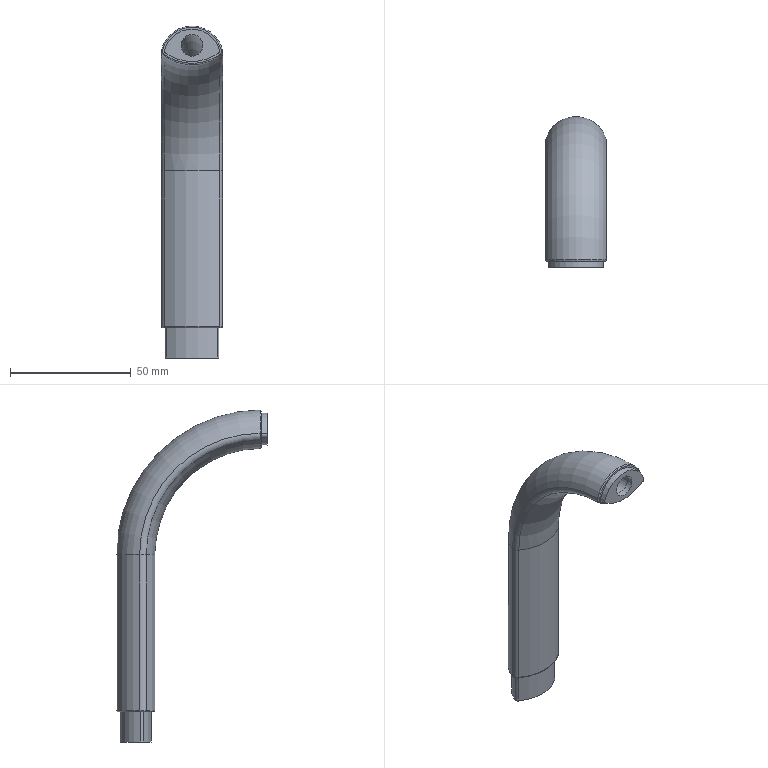Part | NX | features DATUM_CSYS 5, SKETCH 4, BLEND 2, EXTRUDE 2, SCALE 1, SWP104 1 | 1 solid | 31 faces | box 25.275 x 62.5 x 137.498 mm | volume 37253 mm3 | cylinder 14 | torus 9 | plane 4 | spline 4 | commonest cylinder face diameters 2 x2 2.5 x2 5 x2 9 x2 23 x1 23.5 x1
STEP:
#1=CARTESIAN_POINT('',(-12.068,0.2563,0.));
#2=VERTEX_POINT('',#1);
#3=CARTESIAN_POINT('',(12.068,0.2563,0.));
#4=VERTEX_POINT('',#3);
#5=CARTESIAN_POINT('',(0.,-3.,0.));
#6=DIRECTION('',(0.,0.,1.));
#7=DIRECTION('',(1.,0.,0.));
#8=AXIS2_PLACEMENT_3D('',#5,#6,#7);
#9=CIRCLE('',#8,12.5);
#10=EDGE_CURVE('',#2,#4,#9,.F.);
#11=ORIENTED_EDGE('',*,*,#10,.T.);
#12=CARTESIAN_POINT('',(11.296,-1.895,0.));
#13=VERTEX_POINT('',#12);
#14=CARTESIAN_POINT('',(10.137,-0.2647,0.));
#15=DIRECTION('',(0.,0.,1.));
#16=DIRECTION('',(1.,0.,0.));
#17=AXIS2_PLACEMENT_3D('',#14,#15,#16);
#18=CIRCLE('',#17,2.);
#19=EDGE_CURVE('',#4,#13,#18,.F.);
#20=ORIENTED_EDGE('',*,*,#19,.T.);
#21=CARTESIAN_POINT('',(-11.296,-1.895,0.));
#22=VERTEX_POINT('',#21);
#23=CARTESIAN_POINT('',(0.,14.,0.));
#24=DIRECTION('',(0.,0.,1.));
#25=DIRECTION('',(1.,0.,0.));
#26=AXIS2_PLACEMENT_3D('',#23,#24,#25);
#27=CIRCLE('',#26,19.5);
#28=EDGE_CURVE('',#13,#22,#27,.F.);
#29=ORIENTED_EDGE('',*,*,#28,.T.);
#30=CARTESIAN_POINT('',(-10.137,-0.2647,0.));
#31=DIRECTION('',(0.,0.,1.));
#32=DIRECTION('',(1.,0.,0.));
#33=AXIS2_PLACEMENT_3D('',#30,#31,#32);
#34=CIRCLE('',#33,2.);
#35=EDGE_CURVE('',#22,#2,#34,.F.);
#36=ORIENTED_EDGE('',*,*,#35,.T.);
#37=EDGE_LOOP('',(#11,#20,#29,#36));
#38=FACE_BOUND('',#37,.T.);
#39=CARTESIAN_POINT('',(-10.717,-1.08,0.));
#40=VERTEX_POINT('',#39);
#41=CARTESIAN_POINT('',(-11.103,-0.004202,0.));
#42=VERTEX_POINT('',#41);
#43=CARTESIAN_POINT('',(-10.137,-0.2647,0.));
#44=DIRECTION('',(0.,0.,-1.));
#45=DIRECTION('',(1.,0.,0.));
#46=AXIS2_PLACEMENT_3D('',#43,#44,#45);
#47=CIRCLE('',#46,1.);
#48=EDGE_CURVE('',#40,#42,#47,.T.);
#49=ORIENTED_EDGE('',*,*,#48,.F.);
#50=CARTESIAN_POINT('',(10.717,-1.08,0.));
#51=VERTEX_POINT('',#50);
#52=CARTESIAN_POINT('',(0.,14.,0.));
#53=DIRECTION('',(0.,0.,-1.));
#54=DIRECTION('',(1.,0.,0.));
#55=AXIS2_PLACEMENT_3D('',#52,#53,#54);
#56=CIRCLE('',#55,18.5);
#57=EDGE_CURVE('',#51,#40,#56,.T.);
#58=ORIENTED_EDGE('',*,*,#57,.F.);
#59=CARTESIAN_POINT('',(11.103,-0.004202,0.));
#60=VERTEX_POINT('',#59);
#61=CARTESIAN_POINT('',(10.137,-0.2647,0.));
#62=DIRECTION('',(0.,0.,-1.));
#63=DIRECTION('',(1.,0.,0.));
#64=AXIS2_PLACEMENT_3D('',#61,#62,#63);
#65=CIRCLE('',#64,1.);
#66=EDGE_CURVE('',#60,#51,#65,.T.);
#67=ORIENTED_EDGE('',*,*,#66,.F.);
#68=CARTESIAN_POINT('',(0.,-3.,0.));
#69=DIRECTION('',(0.,0.,-1.));
#70=DIRECTION('',(1.,0.,0.));
#71=AXIS2_PLACEMENT_3D('',#68,#69,#70);
#72=CIRCLE('',#71,11.5);
#73=EDGE_CURVE('',#42,#60,#72,.T.);
#74=ORIENTED_EDGE('',*,*,#73,.F.);
#75=EDGE_LOOP('',(#49,#58,#67,#74));
#76=FACE_BOUND('',#75,.T.);
#77=CARTESIAN_POINT('',(5.069,-1.632,0.));
#78=DIRECTION('',(0.,0.,1.));
#79=DIRECTION('',(1.,0.,0.));
#80=AXIS2_PLACEMENT_3D('',#77,#78,#79);
#81=PLANE('',#80);
#82=ADVANCED_FACE('',(#38,#76),#81,.F.);
#83=CARTESIAN_POINT('',(-12.551,0.3866,65.));
#84=VERTEX_POINT('',#83);
#85=CARTESIAN_POINT('',(-12.551,-49.499,115.384));
#86=VERTEX_POINT('',#85);
#87=CARTESIAN_POINT('',(-12.551,-50.,65.));
#88=DIRECTION('',(1.,0.,0.));
#89=DIRECTION('',(0.,0.,-1.));
#90=AXIS2_PLACEMENT_3D('',#87,#88,#89);
#91=CIRCLE('',#90,50.387);
#92=EDGE_CURVE('',#84,#86,#91,.T.);
#93=ORIENTED_EDGE('',*,*,#92,.T.);
#94=CARTESIAN_POINT('',(12.551,-49.499,115.384));
#95=VERTEX_POINT('',#94);
#96=CARTESIAN_POINT('',(-12.551,-49.499,115.384));
#97=CARTESIAN_POINT('',(-11.807,-49.498,118.142));
#98=CARTESIAN_POINT('',(-8.48,-49.496,123.077));
#99=CARTESIAN_POINT('',(-0.002474,-49.496,125.957));
#100=CARTESIAN_POINT('',(8.472,-49.496,123.084));
#101=CARTESIAN_POINT('',(11.807,-49.498,118.142));
#102=CARTESIAN_POINT('',(12.551,-49.499,115.384));
#103=B_SPLINE_CURVE_WITH_KNOTS('',3,(#96,#97,#98,#99,#100,#101,#102),.UNSPECIFIED.,.F.,.F.,(4,1,1,1,4),(0.,0.0085,0.017,0.0255,0.034),.UNSPECIFIED.);
#104=EDGE_CURVE('',#86,#95,#103,.T.);
#105=ORIENTED_EDGE('',*,*,#104,.T.);
#106=CARTESIAN_POINT('',(12.551,0.3866,65.));
#107=VERTEX_POINT('',#106);
#108=CARTESIAN_POINT('',(12.551,-50.,65.));
#109=DIRECTION('',(1.,0.,0.));
#110=DIRECTION('',(0.,0.,-1.));
#111=AXIS2_PLACEMENT_3D('',#108,#109,#110);
#112=CIRCLE('',#111,50.387);
#113=EDGE_CURVE('',#107,#95,#112,.T.);
#114=ORIENTED_EDGE('',*,*,#113,.F.);
#115=CARTESIAN_POINT('',(0.,-3.,65.));
#116=DIRECTION('',(0.,0.,1.));
#117=DIRECTION('',(1.,0.,0.));
#118=AXIS2_PLACEMENT_3D('',#115,#116,#117);
#119=CIRCLE('',#118,13.);
#120=EDGE_CURVE('',#107,#84,#119,.T.);
#121=ORIENTED_EDGE('',*,*,#120,.T.);
#122=EDGE_LOOP('',(#93,#105,#114,#121));
#123=FACE_BOUND('',#122,.T.);
#124=CARTESIAN_POINT('',(0.,-50.,65.));
#125=DIRECTION('',(1.,0.,0.));
#126=DIRECTION('',(0.,0.,-1.));
#127=AXIS2_PLACEMENT_3D('',#124,#125,#126);
#128=TOROIDAL_SURFACE('',#127,47.,13.);
#129=ADVANCED_FACE('',(#123),#128,.T.);
#130=CARTESIAN_POINT('',(-11.586,-2.303,65.));
#131=VERTEX_POINT('',#130);
#132=CARTESIAN_POINT('',(-11.586,-49.504,112.695));
#133=VERTEX_POINT('',#132);
#134=CARTESIAN_POINT('',(-11.586,-50.,65.));
#135=DIRECTION('',(1.,0.,0.));
#136=DIRECTION('',(0.,0.,-1.));
#137=AXIS2_PLACEMENT_3D('',#134,#135,#136);
#138=CIRCLE('',#137,47.697);
#139=EDGE_CURVE('',#131,#133,#138,.T.);
#140=ORIENTED_EDGE('',*,*,#139,.T.);
#141=CARTESIAN_POINT('',(-11.586,-49.504,112.695));
#142=CARTESIAN_POINT('',(-12.419,-49.503,113.287));
#143=CARTESIAN_POINT('',(-12.817,-49.501,114.397));
#144=CARTESIAN_POINT('',(-12.551,-49.499,115.384));
#145=B_SPLINE_CURVE_WITH_KNOTS('',3,(#141,#142,#143,#144),.UNSPECIFIED.,.F.,.F.,(4,4),(0.,0.003051),.UNSPECIFIED.);
#146=EDGE_CURVE('',#133,#86,#145,.T.);
#147=ORIENTED_EDGE('',*,*,#146,.T.);
#148=ORIENTED_EDGE('',*,*,#92,.F.);
#149=CARTESIAN_POINT('',(-10.137,-0.2647,65.));
#150=DIRECTION('',(0.,0.,1.));
#151=DIRECTION('',(1.,0.,0.));
#152=AXIS2_PLACEMENT_3D('',#149,#150,#151);
#153=CIRCLE('',#152,2.5);
#154=EDGE_CURVE('',#84,#131,#153,.T.);
#155=ORIENTED_EDGE('',*,*,#154,.T.);
#156=EDGE_LOOP('',(#140,#147,#148,#155));
#157=FACE_BOUND('',#156,.T.);
#158=CARTESIAN_POINT('',(-10.137,-50.,65.));
#159=DIRECTION('',(1.,0.,0.));
#160=DIRECTION('',(0.,0.,-1.));
#161=AXIS2_PLACEMENT_3D('',#158,#159,#160);
#162=TOROIDAL_SURFACE('',#161,49.735,2.5);
#163=ADVANCED_FACE('',(#157),#162,.T.);
#164=CARTESIAN_POINT('',(11.586,-2.303,65.));
#165=VERTEX_POINT('',#164);
#166=CARTESIAN_POINT('',(11.586,-49.504,112.695));
#167=VERTEX_POINT('',#166);
#168=CARTESIAN_POINT('',(11.586,-50.,65.));
#169=DIRECTION('',(1.,0.,0.));
#170=DIRECTION('',(0.,0.,-1.));
#171=AXIS2_PLACEMENT_3D('',#168,#169,#170);
#172=CIRCLE('',#171,47.697);
#173=EDGE_CURVE('',#165,#167,#172,.T.);
#174=ORIENTED_EDGE('',*,*,#173,.T.);
#175=CARTESIAN_POINT('',(11.586,-49.504,112.695));
#176=CARTESIAN_POINT('',(8.204,-49.505,110.291));
#177=CARTESIAN_POINT('',(-0.002573,-49.506,107.703));
#178=CARTESIAN_POINT('',(-8.204,-49.505,110.291));
#179=CARTESIAN_POINT('',(-11.586,-49.504,112.695));
#180=B_SPLINE_CURVE_WITH_KNOTS('',3,(#175,#176,#177,#178,#179),.UNSPECIFIED.,.F.,.F.,(4,1,4),(0.,0.01237,0.02474),.UNSPECIFIED.);
#181=EDGE_CURVE('',#167,#133,#180,.T.);
#182=ORIENTED_EDGE('',*,*,#181,.T.);
#183=ORIENTED_EDGE('',*,*,#139,.F.);
#184=CARTESIAN_POINT('',(0.,14.,65.));
#185=DIRECTION('',(0.,0.,1.));
#186=DIRECTION('',(1.,0.,0.));
#187=AXIS2_PLACEMENT_3D('',#184,#185,#186);
#188=CIRCLE('',#187,20.);
#189=EDGE_CURVE('',#131,#165,#188,.T.);
#190=ORIENTED_EDGE('',*,*,#189,.T.);
#191=EDGE_LOOP('',(#174,#182,#183,#190));
#192=FACE_BOUND('',#191,.T.);
#193=CARTESIAN_POINT('',(0.,-50.,65.));
#194=DIRECTION('',(1.,0.,0.));
#195=DIRECTION('',(0.,0.,-1.));
#196=AXIS2_PLACEMENT_3D('',#193,#194,#195);
#197=TOROIDAL_SURFACE('',#196,64.,20.);
#198=ADVANCED_FACE('',(#192),#197,.T.);
#199=ORIENTED_EDGE('',*,*,#113,.T.);
#200=CARTESIAN_POINT('',(12.551,-49.499,115.384));
#201=CARTESIAN_POINT('',(12.817,-49.501,114.397));
#202=CARTESIAN_POINT('',(12.419,-49.503,113.287));
#203=CARTESIAN_POINT('',(11.586,-49.504,112.695));
#204=B_SPLINE_CURVE_WITH_KNOTS('',3,(#200,#201,#202,#203),.UNSPECIFIED.,.F.,.F.,(4,4),(0.,0.003051),.UNSPECIFIED.);
#205=EDGE_CURVE('',#95,#167,#204,.T.);
#206=ORIENTED_EDGE('',*,*,#205,.T.);
#207=ORIENTED_EDGE('',*,*,#173,.F.);
#208=CARTESIAN_POINT('',(10.137,-0.2647,65.));
#209=DIRECTION('',(0.,0.,1.));
#210=DIRECTION('',(1.,0.,0.));
#211=AXIS2_PLACEMENT_3D('',#208,#209,#210);
#212=CIRCLE('',#211,2.5);
#213=EDGE_CURVE('',#165,#107,#212,.T.);
#214=ORIENTED_EDGE('',*,*,#213,.T.);
#215=EDGE_LOOP('',(#199,#206,#207,#214));
#216=FACE_BOUND('',#215,.T.);
#217=CARTESIAN_POINT('',(10.137,-50.,65.));
#218=DIRECTION('',(1.,0.,0.));
#219=DIRECTION('',(0.,0.,-1.));
#220=AXIS2_PLACEMENT_3D('',#217,#218,#219);
#221=TOROIDAL_SURFACE('',#220,49.735,2.5);
#222=ADVANCED_FACE('',(#216),#221,.T.);
#223=CARTESIAN_POINT('',(4.5,2.,65.));
#224=VERTEX_POINT('',#223);
#225=CARTESIAN_POINT('',(0.,2.,65.));
#226=DIRECTION('',(0.,0.,1.));
#227=DIRECTION('',(1.,0.,0.));
#228=AXIS2_PLACEMENT_3D('',#225,#226,#227);
#229=CIRCLE('',#228,4.5);
#230=EDGE_CURVE('',#224,#224,#229,.T.);
#231=ORIENTED_EDGE('',*,*,#230,.F.);
#232=EDGE_LOOP('',(#231));
#233=FACE_BOUND('',#232,.T.);
#234=CARTESIAN_POINT('',(4.5,-50.,117.));
#235=VERTEX_POINT('',#234);
#236=CARTESIAN_POINT('',(0.,-50.,117.));
#237=DIRECTION('',(0.,-1.,0.));
#238=DIRECTION('',(1.,0.,0.));
#239=AXIS2_PLACEMENT_3D('',#236,#237,#238);
#240=CIRCLE('',#239,4.5);
#241=EDGE_CURVE('',#235,#235,#240,.T.);
#242=ORIENTED_EDGE('',*,*,#241,.T.);
#243=EDGE_LOOP('',(#242));
#244=FACE_BOUND('',#243,.T.);
#245=CARTESIAN_POINT('',(0.,-50.,65.));
#246=DIRECTION('',(1.,0.,0.));
#247=DIRECTION('',(0.,0.,-1.));
#248=AXIS2_PLACEMENT_3D('',#245,#246,#247);
#249=TOROIDAL_SURFACE('',#248,52.,4.5);
#250=ADVANCED_FACE('',(#233,#244),#249,.F.);
#251=CARTESIAN_POINT('',(11.586,-2.303,0.5));
#252=VERTEX_POINT('',#251);
#253=CARTESIAN_POINT('',(11.586,-2.303,65.));
#254=DIRECTION('',(0.,0.,-1.));
#255=VECTOR('',#254,1000.);
#256=LINE('',#253,#255);
#257=EDGE_CURVE('',#165,#252,#256,.T.);
#258=ORIENTED_EDGE('',*,*,#257,.T.);
#259=CARTESIAN_POINT('',(12.551,0.3866,0.5));
#260=VERTEX_POINT('',#259);
#261=CARTESIAN_POINT('',(10.137,-0.2647,0.5));
#262=DIRECTION('',(0.,0.,1.));
#263=DIRECTION('',(1.,0.,0.));
#264=AXIS2_PLACEMENT_3D('',#261,#262,#263);
#265=CIRCLE('',#264,2.5);
#266=EDGE_CURVE('',#252,#260,#265,.T.);
#267=ORIENTED_EDGE('',*,*,#266,.T.);
#268=CARTESIAN_POINT('',(12.551,0.3866,65.));
#269=DIRECTION('',(0.,0.,-1.));
#270=VECTOR('',#269,1000.);
#271=LINE('',#268,#270);
#272=EDGE_CURVE('',#107,#260,#271,.T.);
#273=ORIENTED_EDGE('',*,*,#272,.F.);
#274=ORIENTED_EDGE('',*,*,#213,.F.);
#275=EDGE_LOOP('',(#258,#267,#273,#274));
#276=FACE_BOUND('',#275,.T.);
#277=CARTESIAN_POINT('',(10.137,-0.2647,65.));
#278=DIRECTION('',(0.,0.,-1.));
#279=DIRECTION('',(-1.,0.,0.));
#280=AXIS2_PLACEMENT_3D('',#277,#278,#279);
#281=CYLINDRICAL_SURFACE('',#280,2.5);
#282=ADVANCED_FACE('',(#276),#281,.T.);
#283=ORIENTED_EDGE('',*,*,#272,.T.);
#284=CARTESIAN_POINT('',(-12.551,0.3866,0.5));
#285=VERTEX_POINT('',#284);
#286=CARTESIAN_POINT('',(0.,-3.,0.5));
#287=DIRECTION('',(0.,0.,1.));
#288=DIRECTION('',(1.,0.,0.));
#289=AXIS2_PLACEMENT_3D('',#286,#287,#288);
#290=CIRCLE('',#289,13.);
#291=EDGE_CURVE('',#260,#285,#290,.T.);
#292=ORIENTED_EDGE('',*,*,#291,.T.);
#293=CARTESIAN_POINT('',(-12.551,0.3866,65.));
#294=DIRECTION('',(0.,0.,-1.));
#295=VECTOR('',#294,1000.);
#296=LINE('',#293,#295);
#297=EDGE_CURVE('',#84,#285,#296,.T.);
#298=ORIENTED_EDGE('',*,*,#297,.F.);
#299=ORIENTED_EDGE('',*,*,#120,.F.);
#300=EDGE_LOOP('',(#283,#292,#298,#299));
#301=FACE_BOUND('',#300,.T.);
#302=CARTESIAN_POINT('',(0.,-3.,65.));
#303=DIRECTION('',(0.,0.,-1.));
#304=DIRECTION('',(-1.,0.,0.));
#305=AXIS2_PLACEMENT_3D('',#302,#303,#304);
#306=CYLINDRICAL_SURFACE('',#305,13.);
#307=ADVANCED_FACE('',(#301),#306,.T.);
#308=ORIENTED_EDGE('',*,*,#297,.T.);
#309=CARTESIAN_POINT('',(-11.586,-2.303,0.5));
#310=VERTEX_POINT('',#309);
#311=CARTESIAN_POINT('',(-10.137,-0.2647,0.5));
#312=DIRECTION('',(0.,0.,1.));
#313=DIRECTION('',(1.,0.,0.));
#314=AXIS2_PLACEMENT_3D('',#311,#312,#313);
#315=CIRCLE('',#314,2.5);
#316=EDGE_CURVE('',#285,#310,#315,.T.);
#317=ORIENTED_EDGE('',*,*,#316,.T.);
#318=CARTESIAN_POINT('',(-11.586,-2.303,65.));
#319=DIRECTION('',(0.,0.,-1.));
#320=VECTOR('',#319,1000.);
#321=LINE('',#318,#320);
#322=EDGE_CURVE('',#131,#310,#321,.T.);
#323=ORIENTED_EDGE('',*,*,#322,.F.);
#324=ORIENTED_EDGE('',*,*,#154,.F.);
#325=EDGE_LOOP('',(#308,#317,#323,#324));
#326=FACE_BOUND('',#325,.T.);
#327=CARTESIAN_POINT('',(-10.137,-0.2647,65.));
#328=DIRECTION('',(0.,0.,-1.));
#329=DIRECTION('',(-1.,0.,0.));
#330=AXIS2_PLACEMENT_3D('',#327,#328,#329);
#331=CYLINDRICAL_SURFACE('',#330,2.5);
#332=ADVANCED_FACE('',(#326),#331,.T.);
#333=ORIENTED_EDGE('',*,*,#230,.T.);
#334=EDGE_LOOP('',(#333));
#335=FACE_BOUND('',#334,.T.);
#336=CARTESIAN_POINT('',(4.5,2.,-12.5));
#337=VERTEX_POINT('',#336);
#338=CARTESIAN_POINT('',(0.,2.,-12.5));
#339=DIRECTION('',(0.,0.,-1.));
#340=DIRECTION('',(1.,0.,0.));
#341=AXIS2_PLACEMENT_3D('',#338,#339,#340);
#342=CIRCLE('',#341,4.5);
#343=EDGE_CURVE('',#337,#337,#342,.T.);
#344=ORIENTED_EDGE('',*,*,#343,.T.);
#345=EDGE_LOOP('',(#344));
#346=FACE_BOUND('',#345,.T.);
#347=CARTESIAN_POINT('',(0.,2.,65.));
#348=DIRECTION('',(0.,0.,-1.));
#349=DIRECTION('',(-1.,0.,0.));
#350=AXIS2_PLACEMENT_3D('',#347,#348,#349);
#351=CYLINDRICAL_SURFACE('',#350,4.5);
#352=ADVANCED_FACE('',(#335,#346),#351,.F.);
#353=ORIENTED_EDGE('',*,*,#322,.T.);
#354=CARTESIAN_POINT('',(0.,14.,0.5));
#355=DIRECTION('',(0.,0.,1.));
#356=DIRECTION('',(1.,0.,0.));
#357=AXIS2_PLACEMENT_3D('',#354,#355,#356);
#358=CIRCLE('',#357,20.);
#359=EDGE_CURVE('',#310,#252,#358,.T.);
#360=ORIENTED_EDGE('',*,*,#359,.T.);
#361=ORIENTED_EDGE('',*,*,#257,.F.);
#362=ORIENTED_EDGE('',*,*,#189,.F.);
#363=EDGE_LOOP('',(#353,#360,#361,#362));
#364=FACE_BOUND('',#363,.T.);
#365=CARTESIAN_POINT('',(0.,14.,65.));
#366=DIRECTION('',(0.,0.,-1.));
#367=DIRECTION('',(-1.,0.,0.));
#368=AXIS2_PLACEMENT_3D('',#365,#366,#367);
#369=CYLINDRICAL_SURFACE('',#368,20.);
#370=ADVANCED_FACE('',(#364),#369,.T.);
#371=CARTESIAN_POINT('',(-11.296,-50.,113.102));
#372=VERTEX_POINT('',#371);
#373=CARTESIAN_POINT('',(11.296,-50.,113.102));
#374=VERTEX_POINT('',#373);
#375=CARTESIAN_POINT('',(-11.296,-50.,113.102));
#376=CARTESIAN_POINT('',(-7.994,-50.,110.756));
#377=CARTESIAN_POINT('',(-0.03503,-50.,108.239));
#378=CARTESIAN_POINT('',(7.994,-50.,110.756));
#379=CARTESIAN_POINT('',(11.296,-50.,113.102));
#380=B_SPLINE_CURVE_WITH_KNOTS('',3,(#375,#376,#377,#378,#379),.UNSPECIFIED.,.F.,.F.,(4,1,4),(0.,0.01198,0.02396),.UNSPECIFIED.);
#381=EDGE_CURVE('',#372,#374,#380,.T.);
#382=ORIENTED_EDGE('',*,*,#381,.T.);
#383=CARTESIAN_POINT('',(12.068,-50.,115.254));
#384=VERTEX_POINT('',#383);
#385=CARTESIAN_POINT('',(11.296,-50.,113.102));
#386=CARTESIAN_POINT('',(11.963,-50.,113.576));
#387=CARTESIAN_POINT('',(12.281,-50.,114.464));
#388=CARTESIAN_POINT('',(12.068,-50.,115.254));
#389=B_SPLINE_CURVE_WITH_KNOTS('',3,(#385,#386,#387,#388),.UNSPECIFIED.,.F.,.F.,(4,4),(0.,0.002419),.UNSPECIFIED.);
#390=EDGE_CURVE('',#374,#384,#389,.T.);
#391=ORIENTED_EDGE('',*,*,#390,.T.);
#392=CARTESIAN_POINT('',(-12.068,-50.,115.254));
#393=VERTEX_POINT('',#392);
#394=CARTESIAN_POINT('',(12.068,-50.,115.254));
#395=CARTESIAN_POINT('',(11.352,-50.,117.907));
#396=CARTESIAN_POINT('',(8.169,-50.,122.635));
#397=CARTESIAN_POINT('',(0.009802,-50.,125.424));
#398=CARTESIAN_POINT('',(-8.149,-50.,122.655));
#399=CARTESIAN_POINT('',(-11.352,-50.,117.907));
#400=CARTESIAN_POINT('',(-12.068,-50.,115.254));
#401=B_SPLINE_CURVE_WITH_KNOTS('',3,(#394,#395,#396,#397,#398,#399,#400),.UNSPECIFIED.,.F.,.F.,(4,1,1,1,4),(0.,0.008128,0.01626,0.02439,0.03251),.UNSPECIFIED.);
#402=EDGE_CURVE('',#384,#393,#401,.T.);
#403=ORIENTED_EDGE('',*,*,#402,.T.);
#404=CARTESIAN_POINT('',(-12.068,-50.,115.254));
#405=CARTESIAN_POINT('',(-12.281,-50.,114.464));
#406=CARTESIAN_POINT('',(-11.963,-50.,113.576));
#407=CARTESIAN_POINT('',(-11.296,-50.,113.102));
#408=B_SPLINE_CURVE_WITH_KNOTS('',3,(#404,#405,#406,#407),.UNSPECIFIED.,.F.,.F.,(4,4),(0.,0.002419),.UNSPECIFIED.);
#409=EDGE_CURVE('',#393,#372,#408,.T.);
#410=ORIENTED_EDGE('',*,*,#409,.T.);
#411=EDGE_LOOP('',(#382,#391,#403,#410));
#412=FACE_BOUND('',#411,.T.);
#413=CARTESIAN_POINT('',(-11.344,-50.,115.061));
#414=VERTEX_POINT('',#413);
#415=CARTESIAN_POINT('',(-10.862,-50.,113.716));
#416=VERTEX_POINT('',#415);
#417=CARTESIAN_POINT('',(-10.137,-50.,114.735));
#418=DIRECTION('',(0.,-1.,0.));
#419=DIRECTION('',(1.,0.,0.));
#420=AXIS2_PLACEMENT_3D('',#417,#418,#419);
#421=CIRCLE('',#420,1.25);
#422=EDGE_CURVE('',#414,#416,#421,.T.);
#423=ORIENTED_EDGE('',*,*,#422,.F.);
#424=CARTESIAN_POINT('',(11.344,-50.,115.061));
#425=VERTEX_POINT('',#424);
#426=CARTESIAN_POINT('',(0.,-50.,112.));
#427=DIRECTION('',(0.,-1.,0.));
#428=DIRECTION('',(1.,0.,0.));
#429=AXIS2_PLACEMENT_3D('',#426,#427,#428);
#430=CIRCLE('',#429,11.75);
#431=EDGE_CURVE('',#425,#414,#430,.T.);
#432=ORIENTED_EDGE('',*,*,#431,.F.);
#433=CARTESIAN_POINT('',(10.862,-50.,113.716));
#434=VERTEX_POINT('',#433);
#435=CARTESIAN_POINT('',(10.137,-50.,114.735));
#436=DIRECTION('',(0.,-1.,0.));
#437=DIRECTION('',(1.,0.,0.));
#438=AXIS2_PLACEMENT_3D('',#435,#436,#437);
#439=CIRCLE('',#438,1.25);
#440=EDGE_CURVE('',#434,#425,#439,.T.);
#441=ORIENTED_EDGE('',*,*,#440,.F.);
#442=CARTESIAN_POINT('',(0.,-50.,129.));
#443=DIRECTION('',(0.,-1.,0.));
#444=DIRECTION('',(1.,0.,0.));
#445=AXIS2_PLACEMENT_3D('',#442,#443,#444);
#446=CIRCLE('',#445,18.75);
#447=EDGE_CURVE('',#416,#434,#446,.T.);
#448=ORIENTED_EDGE('',*,*,#447,.F.);
#449=EDGE_LOOP('',(#423,#432,#441,#448));
#450=FACE_BOUND('',#449,.T.);
#451=CARTESIAN_POINT('',(5.069,-50.,113.368));
#452=DIRECTION('',(0.,-1.,0.));
#453=DIRECTION('',(1.,0.,0.));
#454=AXIS2_PLACEMENT_3D('',#451,#452,#453);
#455=PLANE('',#454);
#456=ADVANCED_FACE('',(#412,#450),#455,.T.);
#457=ORIENTED_EDGE('',*,*,#48,.T.);
#458=CARTESIAN_POINT('',(-11.103,-0.004202,-12.5));
#459=VERTEX_POINT('',#458);
#460=CARTESIAN_POINT('',(-11.103,-0.004202,-12.5));
#461=DIRECTION('',(0.,0.,1.));
#462=VECTOR('',#461,1000.);
#463=LINE('',#460,#462);
#464=EDGE_CURVE('',#459,#42,#463,.T.);
#465=ORIENTED_EDGE('',*,*,#464,.F.);
#466=CARTESIAN_POINT('',(-10.717,-1.08,-12.5));
#467=VERTEX_POINT('',#466);
#468=CARTESIAN_POINT('',(-10.137,-0.2647,-12.5));
#469=DIRECTION('',(0.,0.,-1.));
#470=DIRECTION('',(1.,0.,0.));
#471=AXIS2_PLACEMENT_3D('',#468,#469,#470);
#472=CIRCLE('',#471,1.);
#473=EDGE_CURVE('',#467,#459,#472,.T.);
#474=ORIENTED_EDGE('',*,*,#473,.F.);
#475=CARTESIAN_POINT('',(-10.717,-1.08,-12.5));
#476=DIRECTION('',(0.,0.,1.));
#477=VECTOR('',#476,1000.);
#478=LINE('',#475,#477);
#479=EDGE_CURVE('',#467,#40,#478,.T.);
#480=ORIENTED_EDGE('',*,*,#479,.T.);
#481=EDGE_LOOP('',(#457,#465,#474,#480));
#482=FACE_BOUND('',#481,.T.);
#483=CARTESIAN_POINT('',(-10.137,-0.2647,-12.5));
#484=DIRECTION('',(0.,0.,1.));
#485=DIRECTION('',(1.,0.,0.));
#486=AXIS2_PLACEMENT_3D('',#483,#484,#485);
#487=CYLINDRICAL_SURFACE('',#486,1.);
#488=ADVANCED_FACE('',(#482),#487,.T.);
#489=ORIENTED_EDGE('',*,*,#73,.T.);
#490=CARTESIAN_POINT('',(11.103,-0.004202,-12.5));
#491=VERTEX_POINT('',#490);
#492=CARTESIAN_POINT('',(11.103,-0.004202,-12.5));
#493=DIRECTION('',(0.,0.,1.));
#494=VECTOR('',#493,1000.);
#495=LINE('',#492,#494);
#496=EDGE_CURVE('',#491,#60,#495,.T.);
#497=ORIENTED_EDGE('',*,*,#496,.F.);
#498=CARTESIAN_POINT('',(0.,-3.,-12.5));
#499=DIRECTION('',(0.,0.,-1.));
#500=DIRECTION('',(1.,0.,0.));
#501=AXIS2_PLACEMENT_3D('',#498,#499,#500);
#502=CIRCLE('',#501,11.5);
#503=EDGE_CURVE('',#459,#491,#502,.T.);
#504=ORIENTED_EDGE('',*,*,#503,.F.);
#505=ORIENTED_EDGE('',*,*,#464,.T.);
#506=EDGE_LOOP('',(#489,#497,#504,#505));
#507=FACE_BOUND('',#506,.T.);
#508=CARTESIAN_POINT('',(0.,-3.,-12.5));
#509=DIRECTION('',(0.,0.,1.));
#510=DIRECTION('',(1.,0.,0.));
#511=AXIS2_PLACEMENT_3D('',#508,#509,#510);
#512=CYLINDRICAL_SURFACE('',#511,11.5);
#513=ADVANCED_FACE('',(#507),#512,.T.);
#514=ORIENTED_EDGE('',*,*,#66,.T.);
#515=CARTESIAN_POINT('',(10.717,-1.08,-12.5));
#516=VERTEX_POINT('',#515);
#517=CARTESIAN_POINT('',(10.717,-1.08,-12.5));
#518=DIRECTION('',(0.,0.,1.));
#519=VECTOR('',#518,1000.);
#520=LINE('',#517,#519);
#521=EDGE_CURVE('',#516,#51,#520,.T.);
#522=ORIENTED_EDGE('',*,*,#521,.F.);
#523=CARTESIAN_POINT('',(10.137,-0.2647,-12.5));
#524=DIRECTION('',(0.,0.,-1.));
#525=DIRECTION('',(1.,0.,0.));
#526=AXIS2_PLACEMENT_3D('',#523,#524,#525);
#527=CIRCLE('',#526,1.);
#528=EDGE_CURVE('',#491,#516,#527,.T.);
#529=ORIENTED_EDGE('',*,*,#528,.F.);
#530=ORIENTED_EDGE('',*,*,#496,.T.);
#531=EDGE_LOOP('',(#514,#522,#529,#530));
#532=FACE_BOUND('',#531,.T.);
#533=CARTESIAN_POINT('',(10.137,-0.2647,-12.5));
#534=DIRECTION('',(0.,0.,1.));
#535=DIRECTION('',(1.,0.,0.));
#536=AXIS2_PLACEMENT_3D('',#533,#534,#535);
#537=CYLINDRICAL_SURFACE('',#536,1.);
#538=ADVANCED_FACE('',(#532),#537,.T.);
#539=ORIENTED_EDGE('',*,*,#57,.T.);
#540=ORIENTED_EDGE('',*,*,#479,.F.);
#541=CARTESIAN_POINT('',(0.,14.,-12.5));
#542=DIRECTION('',(0.,0.,-1.));
#543=DIRECTION('',(1.,0.,0.));
#544=AXIS2_PLACEMENT_3D('',#541,#542,#543);
#545=CIRCLE('',#544,18.5);
#546=EDGE_CURVE('',#516,#467,#545,.T.);
#547=ORIENTED_EDGE('',*,*,#546,.F.);
#548=ORIENTED_EDGE('',*,*,#521,.T.);
#549=EDGE_LOOP('',(#539,#540,#547,#548));
#550=FACE_BOUND('',#549,.T.);
#551=CARTESIAN_POINT('',(0.,14.,-12.5));
#552=DIRECTION('',(0.,0.,1.));
#553=DIRECTION('',(1.,0.,0.));
#554=AXIS2_PLACEMENT_3D('',#551,#552,#553);
#555=CYLINDRICAL_SURFACE('',#554,18.5);
#556=ADVANCED_FACE('',(#550),#555,.T.);
#557=ORIENTED_EDGE('',*,*,#473,.T.);
#558=ORIENTED_EDGE('',*,*,#503,.T.);
#559=ORIENTED_EDGE('',*,*,#528,.T.);
#560=ORIENTED_EDGE('',*,*,#546,.T.);
#561=EDGE_LOOP('',(#557,#558,#559,#560));
#562=FACE_BOUND('',#561,.T.);
#563=ORIENTED_EDGE('',*,*,#343,.F.);
#564=EDGE_LOOP('',(#563));
#565=FACE_BOUND('',#564,.T.);
#566=CARTESIAN_POINT('',(-5.069,-1.632,-12.5));
#567=DIRECTION('',(0.,0.,-1.));
#568=DIRECTION('',(-1.,0.,0.));
#569=AXIS2_PLACEMENT_3D('',#566,#567,#568);
#570=PLANE('',#569);
#571=ADVANCED_FACE('',(#562,#565),#570,.T.);
#572=ORIENTED_EDGE('',*,*,#422,.T.);
#573=CARTESIAN_POINT('',(-10.862,-52.5,113.716));
#574=VERTEX_POINT('',#573);
#575=CARTESIAN_POINT('',(-10.862,-52.5,113.716));
#576=DIRECTION('',(0.,1.,0.));
#577=VECTOR('',#576,1000.);
#578=LINE('',#575,#577);
#579=EDGE_CURVE('',#574,#416,#578,.T.);
#580=ORIENTED_EDGE('',*,*,#579,.F.);
#581=CARTESIAN_POINT('',(-11.344,-52.5,115.061));
#582=VERTEX_POINT('',#581);
#583=CARTESIAN_POINT('',(-10.137,-52.5,114.735));
#584=DIRECTION('',(0.,-1.,0.));
#585=DIRECTION('',(1.,0.,0.));
#586=AXIS2_PLACEMENT_3D('',#583,#584,#585);
#587=CIRCLE('',#586,1.25);
#588=EDGE_CURVE('',#582,#574,#587,.T.);
#589=ORIENTED_EDGE('',*,*,#588,.F.);
#590=CARTESIAN_POINT('',(-11.344,-52.5,115.061));
#591=DIRECTION('',(0.,1.,0.));
#592=VECTOR('',#591,1000.);
#593=LINE('',#590,#592);
#594=EDGE_CURVE('',#582,#414,#593,.T.);
#595=ORIENTED_EDGE('',*,*,#594,.T.);
#596=EDGE_LOOP('',(#572,#580,#589,#595));
#597=FACE_BOUND('',#596,.T.);
#598=CARTESIAN_POINT('',(-10.137,-52.5,114.735));
#599=DIRECTION('',(0.,1.,0.));
#600=DIRECTION('',(0.,0.,1.));
#601=AXIS2_PLACEMENT_3D('',#598,#599,#600);
#602=CYLINDRICAL_SURFACE('',#601,1.25);
#603=ADVANCED_FACE('',(#597),#602,.T.);
#604=ORIENTED_EDGE('',*,*,#447,.T.);
#605=CARTESIAN_POINT('',(10.862,-52.5,113.716));
#606=VERTEX_POINT('',#605);
#607=CARTESIAN_POINT('',(10.862,-52.5,113.716));
#608=DIRECTION('',(0.,1.,0.));
#609=VECTOR('',#608,1000.);
#610=LINE('',#607,#609);
#611=EDGE_CURVE('',#606,#434,#610,.T.);
#612=ORIENTED_EDGE('',*,*,#611,.F.);
#613=CARTESIAN_POINT('',(0.,-52.5,129.));
#614=DIRECTION('',(0.,-1.,0.));
#615=DIRECTION('',(1.,0.,0.));
#616=AXIS2_PLACEMENT_3D('',#613,#614,#615);
#617=CIRCLE('',#616,18.75);
#618=EDGE_CURVE('',#574,#606,#617,.T.);
#619=ORIENTED_EDGE('',*,*,#618,.F.);
#620=ORIENTED_EDGE('',*,*,#579,.T.);
#621=EDGE_LOOP('',(#604,#612,#619,#620));
#622=FACE_BOUND('',#621,.T.);
#623=CARTESIAN_POINT('',(0.,-52.5,129.));
#624=DIRECTION('',(0.,1.,0.));
#625=DIRECTION('',(0.,0.,1.));
#626=AXIS2_PLACEMENT_3D('',#623,#624,#625);
#627=CYLINDRICAL_SURFACE('',#626,18.75);
#628=ADVANCED_FACE('',(#622),#627,.T.);
#629=ORIENTED_EDGE('',*,*,#440,.T.);
#630=CARTESIAN_POINT('',(11.344,-52.5,115.061));
#631=VERTEX_POINT('',#630);
#632=CARTESIAN_POINT('',(11.344,-52.5,115.061));
#633=DIRECTION('',(0.,1.,0.));
#634=VECTOR('',#633,1000.);
#635=LINE('',#632,#634);
#636=EDGE_CURVE('',#631,#425,#635,.T.);
#637=ORIENTED_EDGE('',*,*,#636,.F.);
#638=CARTESIAN_POINT('',(10.137,-52.5,114.735));
#639=DIRECTION('',(0.,-1.,0.));
#640=DIRECTION('',(1.,0.,0.));
#641=AXIS2_PLACEMENT_3D('',#638,#639,#640);
#642=CIRCLE('',#641,1.25);
#643=EDGE_CURVE('',#606,#631,#642,.T.);
#644=ORIENTED_EDGE('',*,*,#643,.F.);
#645=ORIENTED_EDGE('',*,*,#611,.T.);
#646=EDGE_LOOP('',(#629,#637,#644,#645));
#647=FACE_BOUND('',#646,.T.);
#648=CARTESIAN_POINT('',(10.137,-52.5,114.735));
#649=DIRECTION('',(0.,1.,0.));
#650=DIRECTION('',(0.,0.,1.));
#651=AXIS2_PLACEMENT_3D('',#648,#649,#650);
#652=CYLINDRICAL_SURFACE('',#651,1.25);
#653=ADVANCED_FACE('',(#647),#652,.T.);
#654=ORIENTED_EDGE('',*,*,#431,.T.);
#655=ORIENTED_EDGE('',*,*,#594,.F.);
#656=CARTESIAN_POINT('',(0.,-52.5,112.));
#657=DIRECTION('',(0.,-1.,0.));
#658=DIRECTION('',(1.,0.,0.));
#659=AXIS2_PLACEMENT_3D('',#656,#657,#658);
#660=CIRCLE('',#659,11.75);
#661=EDGE_CURVE('',#631,#582,#660,.T.);
#662=ORIENTED_EDGE('',*,*,#661,.F.);
#663=ORIENTED_EDGE('',*,*,#636,.T.);
#664=EDGE_LOOP('',(#654,#655,#662,#663));
#665=FACE_BOUND('',#664,.T.);
#666=CARTESIAN_POINT('',(0.,-52.5,112.));
#667=DIRECTION('',(0.,1.,0.));
#668=DIRECTION('',(0.,0.,1.));
#669=AXIS2_PLACEMENT_3D('',#666,#667,#668);
#670=CYLINDRICAL_SURFACE('',#669,11.75);
#671=ADVANCED_FACE('',(#665),#670,.T.);
#672=CARTESIAN_POINT('',(4.5,-52.5,117.));
#673=VERTEX_POINT('',#672);
#674=CARTESIAN_POINT('',(0.,-52.5,117.));
#675=DIRECTION('',(0.,-1.,0.));
#676=DIRECTION('',(1.,0.,0.));
#677=AXIS2_PLACEMENT_3D('',#674,#675,#676);
#678=CIRCLE('',#677,4.5);
#679=EDGE_CURVE('',#673,#673,#678,.T.);
#680=ORIENTED_EDGE('',*,*,#679,.T.);
#681=EDGE_LOOP('',(#680));
#682=FACE_BOUND('',#681,.T.);
#683=ORIENTED_EDGE('',*,*,#241,.F.);
#684=EDGE_LOOP('',(#683));
#685=FACE_BOUND('',#684,.T.);
#686=CARTESIAN_POINT('',(0.,-52.5,117.));
#687=DIRECTION('',(0.,1.,0.));
#688=DIRECTION('',(0.,0.,1.));
#689=AXIS2_PLACEMENT_3D('',#686,#687,#688);
#690=CYLINDRICAL_SURFACE('',#689,4.5);
#691=ADVANCED_FACE('',(#682,#685),#690,.F.);
#692=ORIENTED_EDGE('',*,*,#588,.T.);
#693=ORIENTED_EDGE('',*,*,#618,.T.);
#694=ORIENTED_EDGE('',*,*,#643,.T.);
#695=ORIENTED_EDGE('',*,*,#661,.T.);
#696=EDGE_LOOP('',(#692,#693,#694,#695));
#697=FACE_BOUND('',#696,.T.);
#698=ORIENTED_EDGE('',*,*,#679,.F.);
#699=EDGE_LOOP('',(#698));
#700=FACE_BOUND('',#699,.T.);
#701=CARTESIAN_POINT('',(-5.069,-52.5,121.868));
#702=DIRECTION('',(0.,-1.,0.));
#703=DIRECTION('',(0.,0.,-1.));
#704=AXIS2_PLACEMENT_3D('',#701,#702,#703);
#705=PLANE('',#704);
#706=ADVANCED_FACE('',(#697,#700),#705,.T.);
#707=CARTESIAN_POINT('',(-12.068,-49.5,115.254));
#708=DIRECTION('',(0.2605,0.,0.9655));
#709=DIRECTION('',(0.9655,0.,-0.2605));
#710=AXIS2_PLACEMENT_3D('',#707,#708,#709);
#711=CIRCLE('',#710,0.5);
#712=EDGE_CURVE('',#86,#393,#711,.T.);
#713=ORIENTED_EDGE('',*,*,#712,.F.);
#714=ORIENTED_EDGE('',*,*,#146,.F.);
#715=CARTESIAN_POINT('',(-11.296,-49.5,113.102));
#716=DIRECTION('',(0.8151,0.,-0.5793));
#717=DIRECTION('',(-0.5793,0.,-0.8151));
#718=AXIS2_PLACEMENT_3D('',#715,#716,#717);
#719=CIRCLE('',#718,0.5);
#720=EDGE_CURVE('',#372,#133,#719,.T.);
#721=ORIENTED_EDGE('',*,*,#720,.F.);
#722=ORIENTED_EDGE('',*,*,#409,.F.);
#723=EDGE_LOOP('',(#713,#714,#721,#722));
#724=FACE_BOUND('',#723,.T.);
#725=CARTESIAN_POINT('',(-12.551,-49.499,115.384));
#726=CARTESIAN_POINT('',(-12.552,-50.,115.384));
#727=CARTESIAN_POINT('',(-12.068,-50.,115.254));
#728=CARTESIAN_POINT('',(-12.817,-49.501,114.397));
#729=CARTESIAN_POINT('',(-12.816,-50.,114.398));
#730=CARTESIAN_POINT('',(-12.281,-50.,114.464));
#731=CARTESIAN_POINT('',(-12.419,-49.503,113.287));
#732=CARTESIAN_POINT('',(-12.417,-50.,113.289));
#733=CARTESIAN_POINT('',(-11.963,-50.,113.576));
#734=CARTESIAN_POINT('',(-11.586,-49.504,112.695));
#735=CARTESIAN_POINT('',(-11.583,-50.,112.698));
#736=CARTESIAN_POINT('',(-11.296,-50.,113.102));
#737=(BOUNDED_SURFACE()B_SPLINE_SURFACE(3,2,((#725,#726,#727),(#728,#729,#730),(#731,#732,#733),(#734,#735,#736)),.UNSPECIFIED.,.F.,.F.,.F.)B_SPLINE_SURFACE_WITH_KNOTS((4,4),(3,3),(0.,0.002419),(0.,1.),.PIECEWISE_BEZIER_KNOTS.)GEOMETRIC_REPRESENTATION_ITEM()RATIONAL_B_SPLINE_SURFACE(((1.,0.7062,1.),(1.,0.7076,1.),(1.,0.7092,1.),(1.,0.7101,1.)))REPRESENTATION_ITEM('')SURFACE());
#738=ADVANCED_FACE('',(#724),#737,.T.);
#739=ORIENTED_EDGE('',*,*,#720,.T.);
#740=ORIENTED_EDGE('',*,*,#181,.F.);
#741=CARTESIAN_POINT('',(11.296,-49.5,113.102));
#742=DIRECTION('',(0.8151,0.,0.5793));
#743=DIRECTION('',(0.5793,0.,-0.8151));
#744=AXIS2_PLACEMENT_3D('',#741,#742,#743);
#745=CIRCLE('',#744,0.5);
#746=EDGE_CURVE('',#374,#167,#745,.T.);
#747=ORIENTED_EDGE('',*,*,#746,.F.);
#748=ORIENTED_EDGE('',*,*,#381,.F.);
#749=EDGE_LOOP('',(#739,#740,#747,#748));
#750=FACE_BOUND('',#749,.T.);
#751=CARTESIAN_POINT('',(-11.586,-49.504,112.695));
#752=CARTESIAN_POINT('',(-11.583,-50.,112.698));
#753=CARTESIAN_POINT('',(-11.296,-50.,113.102));
#754=CARTESIAN_POINT('',(-8.199,-49.505,110.288));
#755=CARTESIAN_POINT('',(-8.2,-50.,110.295));
#756=CARTESIAN_POINT('',(-7.994,-50.,110.756));
#757=CARTESIAN_POINT('',(-0.03592,-49.506,107.706));
#758=CARTESIAN_POINT('',(-0.0359,-50.,107.712));
#759=CARTESIAN_POINT('',(-0.03503,-50.,108.239));
#760=CARTESIAN_POINT('',(8.199,-49.505,110.288));
#761=CARTESIAN_POINT('',(8.2,-50.,110.295));
#762=CARTESIAN_POINT('',(7.994,-50.,110.756));
#763=CARTESIAN_POINT('',(11.586,-49.504,112.695));
#764=CARTESIAN_POINT('',(11.583,-50.,112.698));
#765=CARTESIAN_POINT('',(11.296,-50.,113.102));
#766=(BOUNDED_SURFACE()B_SPLINE_SURFACE(3,2,((#751,#752,#753),(#754,#755,#756),(#757,#758,#759),(#760,#761,#762),(#763,#764,#765)),.UNSPECIFIED.,.F.,.F.,.F.)B_SPLINE_SURFACE_WITH_KNOTS((4,1,4),(3,3),(0.,0.01198,0.02396),(0.,1.),.UNSPECIFIED.)GEOMETRIC_REPRESENTATION_ITEM()RATIONAL_B_SPLINE_SURFACE(((1.,0.7101,1.),(1.,0.7107,1.),(1.,0.7115,1.),(1.,0.7107,1.),(1.,0.7101,1.)))REPRESENTATION_ITEM('')SURFACE());
#767=ADVANCED_FACE('',(#750),#766,.T.);
#768=ORIENTED_EDGE('',*,*,#712,.T.);
#769=ORIENTED_EDGE('',*,*,#402,.F.);
#770=CARTESIAN_POINT('',(12.068,-49.5,115.254));
#771=DIRECTION('',(0.2605,0.,-0.9655));
#772=DIRECTION('',(-0.9655,0.,-0.2605));
#773=AXIS2_PLACEMENT_3D('',#770,#771,#772);
#774=CIRCLE('',#773,0.5);
#775=EDGE_CURVE('',#95,#384,#774,.T.);
#776=ORIENTED_EDGE('',*,*,#775,.F.);
#777=ORIENTED_EDGE('',*,*,#104,.F.);
#778=EDGE_LOOP('',(#768,#769,#776,#777));
#779=FACE_BOUND('',#778,.T.);
#780=CARTESIAN_POINT('',(12.551,-49.499,115.384));
#781=CARTESIAN_POINT('',(12.552,-50.,115.384));
#782=CARTESIAN_POINT('',(12.068,-50.,115.254));
#783=CARTESIAN_POINT('',(11.807,-49.498,118.144));
#784=CARTESIAN_POINT('',(11.808,-50.,118.147));
#785=CARTESIAN_POINT('',(11.352,-50.,117.907));
#786=CARTESIAN_POINT('',(8.496,-49.496,123.06));
#787=CARTESIAN_POINT('',(8.495,-50.,123.066));
#788=CARTESIAN_POINT('',(8.169,-50.,122.635));
#789=CARTESIAN_POINT('',(0.01019,-49.496,125.961));
#790=CARTESIAN_POINT('',(0.01018,-50.,125.966));
#791=CARTESIAN_POINT('',(0.009802,-50.,125.424));
#792=CARTESIAN_POINT('',(-8.475,-49.496,123.081));
#793=CARTESIAN_POINT('',(-8.474,-50.,123.087));
#794=CARTESIAN_POINT('',(-8.149,-50.,122.655));
#795=CARTESIAN_POINT('',(-11.807,-49.498,118.144));
#796=CARTESIAN_POINT('',(-11.808,-50.,118.147));
#797=CARTESIAN_POINT('',(-11.352,-50.,117.907));
#798=CARTESIAN_POINT('',(-12.551,-49.499,115.384));
#799=CARTESIAN_POINT('',(-12.552,-50.,115.384));
#800=CARTESIAN_POINT('',(-12.068,-50.,115.254));
#801=(BOUNDED_SURFACE()B_SPLINE_SURFACE(3,2,((#780,#781,#782),(#783,#784,#785),(#786,#787,#788),(#789,#790,#791),(#792,#793,#794),(#795,#796,#797),(#798,#799,#800)),.UNSPECIFIED.,.F.,.F.,.F.)B_SPLINE_SURFACE_WITH_KNOTS((4,1,1,1,4),(3,3),(0.,0.008128,0.01626,0.02439,0.03251),(0.,1.),.UNSPECIFIED.)GEOMETRIC_REPRESENTATION_ITEM()RATIONAL_B_SPLINE_SURFACE(((1.,0.7062,1.),(1.,0.7055,1.),(1.,0.7045,1.),(1.,0.704,1.),(1.,0.7045,1.),(1.,0.7055,1.),(1.,0.7062,1.)))REPRESENTATION_ITEM('')SURFACE());
#802=ADVANCED_FACE('',(#779),#801,.T.);
#803=ORIENTED_EDGE('',*,*,#746,.T.);
#804=ORIENTED_EDGE('',*,*,#205,.F.);
#805=ORIENTED_EDGE('',*,*,#775,.T.);
#806=ORIENTED_EDGE('',*,*,#390,.F.);
#807=EDGE_LOOP('',(#803,#804,#805,#806));
#808=FACE_BOUND('',#807,.T.);
#809=CARTESIAN_POINT('',(11.586,-49.504,112.695));
#810=CARTESIAN_POINT('',(11.583,-50.,112.698));
#811=CARTESIAN_POINT('',(11.296,-50.,113.102));
#812=CARTESIAN_POINT('',(12.419,-49.503,113.287));
#813=CARTESIAN_POINT('',(12.417,-50.,113.289));
#814=CARTESIAN_POINT('',(11.963,-50.,113.576));
#815=CARTESIAN_POINT('',(12.817,-49.501,114.397));
#816=CARTESIAN_POINT('',(12.816,-50.,114.398));
#817=CARTESIAN_POINT('',(12.281,-50.,114.464));
#818=CARTESIAN_POINT('',(12.551,-49.499,115.384));
#819=CARTESIAN_POINT('',(12.552,-50.,115.384));
#820=CARTESIAN_POINT('',(12.068,-50.,115.254));
#821=(BOUNDED_SURFACE()B_SPLINE_SURFACE(3,2,((#809,#810,#811),(#812,#813,#814),(#815,#816,#817),(#818,#819,#820)),.UNSPECIFIED.,.F.,.F.,.F.)B_SPLINE_SURFACE_WITH_KNOTS((4,4),(3,3),(0.,0.002419),(0.,1.),.PIECEWISE_BEZIER_KNOTS.)GEOMETRIC_REPRESENTATION_ITEM()RATIONAL_B_SPLINE_SURFACE(((1.,0.7101,1.),(1.,0.7092,1.),(1.,0.7076,1.),(1.,0.7062,1.)))REPRESENTATION_ITEM('')SURFACE());
#822=ADVANCED_FACE('',(#808),#821,.T.);
#823=CARTESIAN_POINT('',(-12.068,0.2563,0.5));
#824=DIRECTION('',(0.2605,0.9655,0.));
#825=DIRECTION('',(-0.9655,0.2605,0.));
#826=AXIS2_PLACEMENT_3D('',#823,#824,#825);
#827=CIRCLE('',#826,0.5);
#828=EDGE_CURVE('',#2,#285,#827,.T.);
#829=ORIENTED_EDGE('',*,*,#828,.F.);
#830=ORIENTED_EDGE('',*,*,#35,.F.);
#831=CARTESIAN_POINT('',(-11.296,-1.895,0.5));
#832=DIRECTION('',(0.8151,-0.5793,0.));
#833=DIRECTION('',(0.5793,0.8151,0.));
#834=AXIS2_PLACEMENT_3D('',#831,#832,#833);
#835=CIRCLE('',#834,0.5);
#836=EDGE_CURVE('',#310,#22,#835,.T.);
#837=ORIENTED_EDGE('',*,*,#836,.F.);
#838=ORIENTED_EDGE('',*,*,#316,.F.);
#839=EDGE_LOOP('',(#829,#830,#837,#838));
#840=FACE_BOUND('',#839,.T.);
#841=CARTESIAN_POINT('',(-10.137,-0.2647,0.5));
#842=DIRECTION('',(0.,0.,1.));
#843=DIRECTION('',(1.,0.,0.));
#844=AXIS2_PLACEMENT_3D('',#841,#842,#843);
#845=TOROIDAL_SURFACE('',#844,2.,0.5);
#846=ADVANCED_FACE('',(#840),#845,.T.);
#847=ORIENTED_EDGE('',*,*,#836,.T.);
#848=ORIENTED_EDGE('',*,*,#28,.F.);
#849=CARTESIAN_POINT('',(11.296,-1.895,0.5));
#850=DIRECTION('',(0.8151,0.5793,0.));
#851=DIRECTION('',(-0.5793,0.8151,0.));
#852=AXIS2_PLACEMENT_3D('',#849,#850,#851);
#853=CIRCLE('',#852,0.5);
#854=EDGE_CURVE('',#252,#13,#853,.T.);
#855=ORIENTED_EDGE('',*,*,#854,.F.);
#856=ORIENTED_EDGE('',*,*,#359,.F.);
#857=EDGE_LOOP('',(#847,#848,#855,#856));
#858=FACE_BOUND('',#857,.T.);
#859=CARTESIAN_POINT('',(0.,14.,0.5));
#860=DIRECTION('',(0.,0.,1.));
#861=DIRECTION('',(1.,0.,0.));
#862=AXIS2_PLACEMENT_3D('',#859,#860,#861);
#863=TOROIDAL_SURFACE('',#862,19.5,0.5);
#864=ADVANCED_FACE('',(#858),#863,.T.);
#865=ORIENTED_EDGE('',*,*,#828,.T.);
#866=ORIENTED_EDGE('',*,*,#291,.F.);
#867=CARTESIAN_POINT('',(12.068,0.2563,0.5));
#868=DIRECTION('',(0.2605,-0.9655,0.));
#869=DIRECTION('',(0.9655,0.2605,0.));
#870=AXIS2_PLACEMENT_3D('',#867,#868,#869);
#871=CIRCLE('',#870,0.5);
#872=EDGE_CURVE('',#4,#260,#871,.T.);
#873=ORIENTED_EDGE('',*,*,#872,.F.);
#874=ORIENTED_EDGE('',*,*,#10,.F.);
#875=EDGE_LOOP('',(#865,#866,#873,#874));
#876=FACE_BOUND('',#875,.T.);
#877=CARTESIAN_POINT('',(0.,-3.,0.5));
#878=DIRECTION('',(0.,0.,1.));
#879=DIRECTION('',(1.,0.,0.));
#880=AXIS2_PLACEMENT_3D('',#877,#878,#879);
#881=TOROIDAL_SURFACE('',#880,12.5,0.5);
#882=ADVANCED_FACE('',(#876),#881,.T.);
#883=ORIENTED_EDGE('',*,*,#854,.T.);
#884=ORIENTED_EDGE('',*,*,#19,.F.);
#885=ORIENTED_EDGE('',*,*,#872,.T.);
#886=ORIENTED_EDGE('',*,*,#266,.F.);
#887=EDGE_LOOP('',(#883,#884,#885,#886));
#888=FACE_BOUND('',#887,.T.);
#889=CARTESIAN_POINT('',(10.137,-0.2647,0.5));
#890=DIRECTION('',(0.,0.,1.));
#891=DIRECTION('',(1.,0.,0.));
#892=AXIS2_PLACEMENT_3D('',#889,#890,#891);
#893=TOROIDAL_SURFACE('',#892,2.,0.5);
#894=ADVANCED_FACE('',(#888),#893,.T.);
#895=CLOSED_SHELL('',(#82,#129,#163,#198,#222,#250,#282,#307,#332,#352,#370,#456,#488,#513,#538,#556,#571,#603,#628,#653,#671,#691,#706,#738,#767,#802,#822,#846,#864,#882,#894));
#896=MANIFOLD_SOLID_BREP('',#895);
#897=(LENGTH_UNIT()NAMED_UNIT(*)SI_UNIT(.MILLI.,.METRE.));
#898=UNCERTAINTY_MEASURE_WITH_UNIT(LENGTH_MEASURE(0.0508),#897,'','');
#899=(NAMED_UNIT(*)PLANE_ANGLE_UNIT()SI_UNIT($,.RADIAN.));
#900=(NAMED_UNIT(*)SI_UNIT($,.STERADIAN.)SOLID_ANGLE_UNIT());
#901=(GEOMETRIC_REPRESENTATION_CONTEXT(3)GLOBAL_UNCERTAINTY_ASSIGNED_CONTEXT((#898))GLOBAL_UNIT_ASSIGNED_CONTEXT((#897,#899,#900))REPRESENTATION_CONTEXT('',''));
#902=ADVANCED_BREP_SHAPE_REPRESENTATION('',(#896),#901);